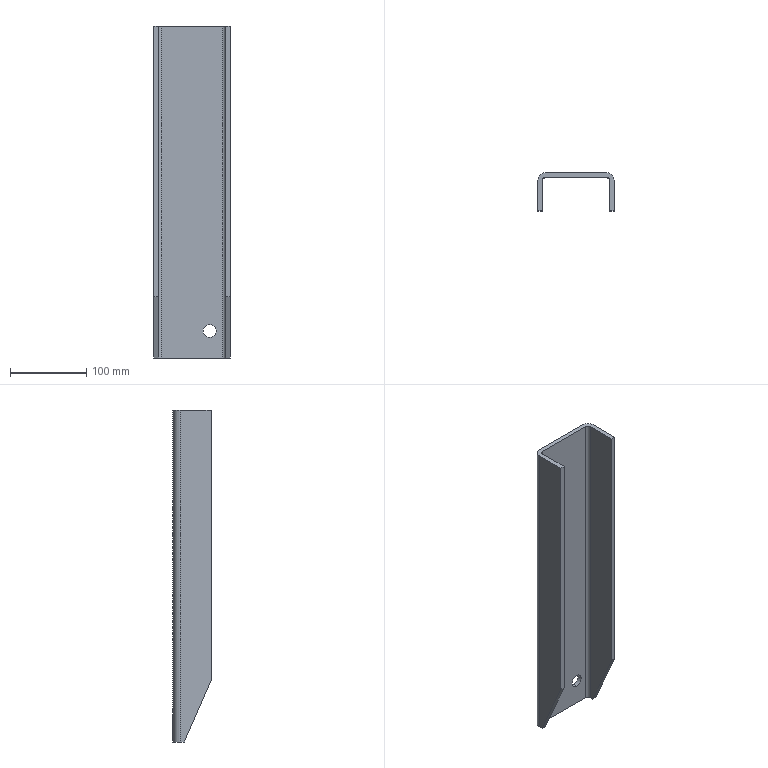Part | SolidWorks | features ICE 2, Extrusion 1 | 1 solid | 18 faces | box 100 x 50 x 435 mm | volume 456835 mm3 | plane 12 | cylinder 6 | commonest cylinder face diameters 8 x2 17 x2 20 x2
STEP:
#1=CARTESIAN_POINT('',(73.2,44.,27.));
#2=VERTEX_POINT('',#1);
#3=CARTESIAN_POINT('',(73.2,44.,44.));
#4=VERTEX_POINT('',#3);
#5=CARTESIAN_POINT('',(73.2,44.,35.5));
#6=DIRECTION('',(0.,1.,0.));
#7=DIRECTION('',(-1.,0.,0.));
#8=AXIS2_PLACEMENT_3D('',#5,#6,#7);
#9=CIRCLE('',#8,8.5);
#10=EDGE_CURVE('',#2,#4,#9,.T.);
#11=ORIENTED_EDGE('',*,*,#10,.F.);
#12=CARTESIAN_POINT('',(73.2,50.,27.));
#13=VERTEX_POINT('',#12);
#14=CARTESIAN_POINT('',(73.2,-385.,27.));
#15=DIRECTION('',(0.,1.,0.));
#16=VECTOR('',#15,1000.);
#17=LINE('',#14,#16);
#18=EDGE_CURVE('',#2,#13,#17,.T.);
#19=ORIENTED_EDGE('',*,*,#18,.T.);
#20=CARTESIAN_POINT('',(73.2,50.,44.));
#21=VERTEX_POINT('',#20);
#22=CARTESIAN_POINT('',(73.2,50.,35.5));
#23=DIRECTION('',(0.,1.,0.));
#24=DIRECTION('',(0.,0.,1.));
#25=AXIS2_PLACEMENT_3D('',#22,#23,#24);
#26=CIRCLE('',#25,8.5);
#27=EDGE_CURVE('',#13,#21,#26,.T.);
#28=ORIENTED_EDGE('',*,*,#27,.T.);
#29=CARTESIAN_POINT('',(73.2,-385.,44.));
#30=DIRECTION('',(0.,1.,0.));
#31=VECTOR('',#30,1000.);
#32=LINE('',#29,#31);
#33=EDGE_CURVE('',#4,#21,#32,.T.);
#34=ORIENTED_EDGE('',*,*,#33,.F.);
#35=EDGE_LOOP('',(#11,#19,#28,#34));
#36=FACE_OUTER_BOUND('',#35,.T.);
#37=CARTESIAN_POINT('',(73.2,-385.,35.5));
#38=DIRECTION('',(0.,1.,0.));
#39=DIRECTION('',(0.,0.,1.));
#40=AXIS2_PLACEMENT_3D('',#37,#38,#39);
#41=CYLINDRICAL_SURFACE('',#40,8.5);
#42=ADVANCED_FACE('',(#36),#41,.F.);
#43=CARTESIAN_POINT('',(100.,35.,0.));
#44=VERTEX_POINT('',#43);
#45=CARTESIAN_POINT('',(100.,0.,80.));
#46=VERTEX_POINT('',#45);
#47=CARTESIAN_POINT('',(100.,0.,80.));
#48=DIRECTION('',(0.,-0.4008,0.9162));
#49=VECTOR('',#48,1000.);
#50=LINE('',#47,#49);
#51=EDGE_CURVE('',#44,#46,#50,.T.);
#52=ORIENTED_EDGE('',*,*,#51,.F.);
#53=CARTESIAN_POINT('',(100.,40.,0.));
#54=VERTEX_POINT('',#53);
#55=CARTESIAN_POINT('',(100.,40.,0.));
#56=DIRECTION('',(0.,-1.,0.));
#57=VECTOR('',#56,1000.);
#58=LINE('',#55,#57);
#59=EDGE_CURVE('',#54,#44,#58,.T.);
#60=ORIENTED_EDGE('',*,*,#59,.F.);
#61=CARTESIAN_POINT('',(100.,40.,435.));
#62=VERTEX_POINT('',#61);
#63=CARTESIAN_POINT('',(100.,40.,435.));
#64=DIRECTION('',(0.,0.,-1.));
#65=VECTOR('',#64,1000.);
#66=LINE('',#63,#65);
#67=EDGE_CURVE('',#62,#54,#66,.T.);
#68=ORIENTED_EDGE('',*,*,#67,.F.);
#69=CARTESIAN_POINT('',(100.,0.,435.));
#70=VERTEX_POINT('',#69);
#71=CARTESIAN_POINT('',(100.,40.,435.));
#72=DIRECTION('',(0.,-1.,0.));
#73=VECTOR('',#72,1000.);
#74=LINE('',#71,#73);
#75=EDGE_CURVE('',#62,#70,#74,.T.);
#76=ORIENTED_EDGE('',*,*,#75,.T.);
#77=CARTESIAN_POINT('',(100.,0.,435.));
#78=DIRECTION('',(0.,0.,-1.));
#79=VECTOR('',#78,1000.);
#80=LINE('',#77,#79);
#81=EDGE_CURVE('',#70,#46,#80,.T.);
#82=ORIENTED_EDGE('',*,*,#81,.T.);
#83=EDGE_LOOP('',(#52,#60,#68,#76,#82));
#84=FACE_OUTER_BOUND('',#83,.T.);
#85=CARTESIAN_POINT('',(100.,40.,435.));
#86=DIRECTION('',(1.,0.,0.));
#87=DIRECTION('',(0.,0.,-1.));
#88=AXIS2_PLACEMENT_3D('',#85,#86,#87);
#89=PLANE('',#88);
#90=ADVANCED_FACE('',(#84),#89,.T.);
#91=CARTESIAN_POINT('',(90.,50.,0.));
#92=VERTEX_POINT('',#91);
#93=CARTESIAN_POINT('',(90.,40.,0.));
#94=DIRECTION('',(0.,0.,-1.));
#95=DIRECTION('',(-1.,0.,0.));
#96=AXIS2_PLACEMENT_3D('',#93,#94,#95);
#97=CIRCLE('',#96,10.);
#98=EDGE_CURVE('',#92,#54,#97,.T.);
#99=ORIENTED_EDGE('',*,*,#98,.F.);
#100=CARTESIAN_POINT('',(90.,50.,435.));
#101=VERTEX_POINT('',#100);
#102=CARTESIAN_POINT('',(90.,50.,435.));
#103=DIRECTION('',(0.,0.,-1.));
#104=VECTOR('',#103,1000.);
#105=LINE('',#102,#104);
#106=EDGE_CURVE('',#101,#92,#105,.T.);
#107=ORIENTED_EDGE('',*,*,#106,.F.);
#108=CARTESIAN_POINT('',(90.,40.,435.));
#109=DIRECTION('',(0.,0.,-1.));
#110=DIRECTION('',(-1.,0.,0.));
#111=AXIS2_PLACEMENT_3D('',#108,#109,#110);
#112=CIRCLE('',#111,10.);
#113=EDGE_CURVE('',#101,#62,#112,.T.);
#114=ORIENTED_EDGE('',*,*,#113,.T.);
#115=ORIENTED_EDGE('',*,*,#67,.T.);
#116=EDGE_LOOP('',(#99,#107,#114,#115));
#117=FACE_OUTER_BOUND('',#116,.T.);
#118=CARTESIAN_POINT('',(90.,40.,435.));
#119=DIRECTION('',(0.,0.,-1.));
#120=DIRECTION('',(-1.,0.,0.));
#121=AXIS2_PLACEMENT_3D('',#118,#119,#120);
#122=CYLINDRICAL_SURFACE('',#121,10.);
#123=ADVANCED_FACE('',(#117),#122,.T.);
#124=CARTESIAN_POINT('',(73.2,50.,35.5));
#125=DIRECTION('',(0.,1.,0.));
#126=DIRECTION('',(0.,0.,1.));
#127=AXIS2_PLACEMENT_3D('',#124,#125,#126);
#128=CIRCLE('',#127,8.5);
#129=EDGE_CURVE('',#21,#13,#128,.T.);
#130=ORIENTED_EDGE('',*,*,#129,.F.);
#131=ORIENTED_EDGE('',*,*,#27,.F.);
#132=EDGE_LOOP('',(#130,#131));
#133=FACE_BOUND('',#132,.T.);
#134=CARTESIAN_POINT('',(10.,50.,0.));
#135=VERTEX_POINT('',#134);
#136=CARTESIAN_POINT('',(10.,50.,0.));
#137=DIRECTION('',(1.,0.,0.));
#138=VECTOR('',#137,1000.);
#139=LINE('',#136,#138);
#140=EDGE_CURVE('',#135,#92,#139,.T.);
#141=ORIENTED_EDGE('',*,*,#140,.F.);
#142=CARTESIAN_POINT('',(10.,50.,435.));
#143=VERTEX_POINT('',#142);
#144=CARTESIAN_POINT('',(10.,50.,435.));
#145=DIRECTION('',(0.,0.,-1.));
#146=VECTOR('',#145,1000.);
#147=LINE('',#144,#146);
#148=EDGE_CURVE('',#143,#135,#147,.T.);
#149=ORIENTED_EDGE('',*,*,#148,.F.);
#150=CARTESIAN_POINT('',(10.,50.,435.));
#151=DIRECTION('',(1.,0.,0.));
#152=VECTOR('',#151,1000.);
#153=LINE('',#150,#152);
#154=EDGE_CURVE('',#143,#101,#153,.T.);
#155=ORIENTED_EDGE('',*,*,#154,.T.);
#156=ORIENTED_EDGE('',*,*,#106,.T.);
#157=EDGE_LOOP('',(#141,#149,#155,#156));
#158=FACE_OUTER_BOUND('',#157,.T.);
#159=CARTESIAN_POINT('',(10.,50.,435.));
#160=DIRECTION('',(0.,1.,0.));
#161=DIRECTION('',(0.,0.,1.));
#162=AXIS2_PLACEMENT_3D('',#159,#160,#161);
#163=PLANE('',#162);
#164=ADVANCED_FACE('',(#133,#158),#163,.T.);
#165=CARTESIAN_POINT('',(0.,40.,0.));
#166=VERTEX_POINT('',#165);
#167=CARTESIAN_POINT('',(10.,40.,0.));
#168=DIRECTION('',(0.,0.,-1.));
#169=DIRECTION('',(-1.,0.,0.));
#170=AXIS2_PLACEMENT_3D('',#167,#168,#169);
#171=CIRCLE('',#170,10.);
#172=EDGE_CURVE('',#166,#135,#171,.T.);
#173=ORIENTED_EDGE('',*,*,#172,.F.);
#174=CARTESIAN_POINT('',(0.,40.,435.));
#175=VERTEX_POINT('',#174);
#176=CARTESIAN_POINT('',(0.,40.,435.));
#177=DIRECTION('',(0.,0.,-1.));
#178=VECTOR('',#177,1000.);
#179=LINE('',#176,#178);
#180=EDGE_CURVE('',#175,#166,#179,.T.);
#181=ORIENTED_EDGE('',*,*,#180,.F.);
#182=CARTESIAN_POINT('',(10.,40.,435.));
#183=DIRECTION('',(0.,0.,-1.));
#184=DIRECTION('',(-1.,0.,0.));
#185=AXIS2_PLACEMENT_3D('',#182,#183,#184);
#186=CIRCLE('',#185,10.);
#187=EDGE_CURVE('',#175,#143,#186,.T.);
#188=ORIENTED_EDGE('',*,*,#187,.T.);
#189=ORIENTED_EDGE('',*,*,#148,.T.);
#190=EDGE_LOOP('',(#173,#181,#188,#189));
#191=FACE_OUTER_BOUND('',#190,.T.);
#192=CARTESIAN_POINT('',(10.,40.,435.));
#193=DIRECTION('',(0.,0.,-1.));
#194=DIRECTION('',(-1.,0.,0.));
#195=AXIS2_PLACEMENT_3D('',#192,#193,#194);
#196=CYLINDRICAL_SURFACE('',#195,10.);
#197=ADVANCED_FACE('',(#191),#196,.T.);
#198=CARTESIAN_POINT('',(0.,0.,80.));
#199=VERTEX_POINT('',#198);
#200=CARTESIAN_POINT('',(0.,35.,0.));
#201=VERTEX_POINT('',#200);
#202=CARTESIAN_POINT('',(0.,-130.361,377.967));
#203=DIRECTION('',(0.,0.4008,-0.9162));
#204=VECTOR('',#203,1000.);
#205=LINE('',#202,#204);
#206=EDGE_CURVE('',#199,#201,#205,.T.);
#207=ORIENTED_EDGE('',*,*,#206,.F.);
#208=CARTESIAN_POINT('',(0.,0.,435.));
#209=VERTEX_POINT('',#208);
#210=CARTESIAN_POINT('',(0.,0.,435.));
#211=DIRECTION('',(0.,0.,-1.));
#212=VECTOR('',#211,1000.);
#213=LINE('',#210,#212);
#214=EDGE_CURVE('',#209,#199,#213,.T.);
#215=ORIENTED_EDGE('',*,*,#214,.F.);
#216=CARTESIAN_POINT('',(0.,0.,435.));
#217=DIRECTION('',(0.,1.,0.));
#218=VECTOR('',#217,1000.);
#219=LINE('',#216,#218);
#220=EDGE_CURVE('',#209,#175,#219,.T.);
#221=ORIENTED_EDGE('',*,*,#220,.T.);
#222=ORIENTED_EDGE('',*,*,#180,.T.);
#223=CARTESIAN_POINT('',(0.,0.,0.));
#224=DIRECTION('',(0.,1.,0.));
#225=VECTOR('',#224,1000.);
#226=LINE('',#223,#225);
#227=EDGE_CURVE('',#201,#166,#226,.T.);
#228=ORIENTED_EDGE('',*,*,#227,.F.);
#229=EDGE_LOOP('',(#207,#215,#221,#222,#228));
#230=FACE_OUTER_BOUND('',#229,.T.);
#231=CARTESIAN_POINT('',(0.,0.,435.));
#232=DIRECTION('',(-1.,0.,0.));
#233=DIRECTION('',(0.,-1.,0.));
#234=AXIS2_PLACEMENT_3D('',#231,#232,#233);
#235=PLANE('',#234);
#236=ADVANCED_FACE('',(#230),#235,.T.);
#237=CARTESIAN_POINT('',(6.,0.,80.));
#238=VERTEX_POINT('',#237);
#239=CARTESIAN_POINT('',(-335.,0.,80.));
#240=DIRECTION('',(1.,0.,0.));
#241=VECTOR('',#240,1000.);
#242=LINE('',#239,#241);
#243=EDGE_CURVE('',#199,#238,#242,.T.);
#244=ORIENTED_EDGE('',*,*,#243,.T.);
#245=CARTESIAN_POINT('',(6.,0.,435.));
#246=VERTEX_POINT('',#245);
#247=CARTESIAN_POINT('',(6.,0.,435.));
#248=DIRECTION('',(0.,0.,-1.));
#249=VECTOR('',#248,1000.);
#250=LINE('',#247,#249);
#251=EDGE_CURVE('',#246,#238,#250,.T.);
#252=ORIENTED_EDGE('',*,*,#251,.F.);
#253=CARTESIAN_POINT('',(6.,0.,435.));
#254=DIRECTION('',(-1.,0.,0.));
#255=VECTOR('',#254,1000.);
#256=LINE('',#253,#255);
#257=EDGE_CURVE('',#246,#209,#256,.T.);
#258=ORIENTED_EDGE('',*,*,#257,.T.);
#259=ORIENTED_EDGE('',*,*,#214,.T.);
#260=EDGE_LOOP('',(#244,#252,#258,#259));
#261=FACE_OUTER_BOUND('',#260,.T.);
#262=CARTESIAN_POINT('',(6.,0.,435.));
#263=DIRECTION('',(0.,-1.,0.));
#264=DIRECTION('',(1.,0.,0.));
#265=AXIS2_PLACEMENT_3D('',#262,#263,#264);
#266=PLANE('',#265);
#267=ADVANCED_FACE('',(#261),#266,.T.);
#268=ORIENTED_EDGE('',*,*,#251,.T.);
#269=CARTESIAN_POINT('',(6.,35.,0.));
#270=VERTEX_POINT('',#269);
#271=CARTESIAN_POINT('',(6.,-130.361,377.967));
#272=DIRECTION('',(0.,0.4008,-0.9162));
#273=VECTOR('',#272,1000.);
#274=LINE('',#271,#273);
#275=EDGE_CURVE('',#238,#270,#274,.T.);
#276=ORIENTED_EDGE('',*,*,#275,.T.);
#277=CARTESIAN_POINT('',(6.,40.,0.));
#278=VERTEX_POINT('',#277);
#279=CARTESIAN_POINT('',(6.,0.,0.));
#280=DIRECTION('',(0.,1.,0.));
#281=VECTOR('',#280,1000.);
#282=LINE('',#279,#281);
#283=EDGE_CURVE('',#270,#278,#282,.T.);
#284=ORIENTED_EDGE('',*,*,#283,.T.);
#285=CARTESIAN_POINT('',(6.,40.,435.));
#286=VERTEX_POINT('',#285);
#287=CARTESIAN_POINT('',(6.,40.,435.));
#288=DIRECTION('',(0.,0.,-1.));
#289=VECTOR('',#288,1000.);
#290=LINE('',#287,#289);
#291=EDGE_CURVE('',#286,#278,#290,.T.);
#292=ORIENTED_EDGE('',*,*,#291,.F.);
#293=CARTESIAN_POINT('',(6.,0.,435.));
#294=DIRECTION('',(0.,1.,0.));
#295=VECTOR('',#294,1000.);
#296=LINE('',#293,#295);
#297=EDGE_CURVE('',#246,#286,#296,.T.);
#298=ORIENTED_EDGE('',*,*,#297,.F.);
#299=EDGE_LOOP('',(#268,#276,#284,#292,#298));
#300=FACE_OUTER_BOUND('',#299,.T.);
#301=CARTESIAN_POINT('',(6.,0.,435.));
#302=DIRECTION('',(-1.,0.,0.));
#303=DIRECTION('',(0.,-1.,0.));
#304=AXIS2_PLACEMENT_3D('',#301,#302,#303);
#305=PLANE('',#304);
#306=ADVANCED_FACE('',(#300),#305,.F.);
#307=CARTESIAN_POINT('',(10.,44.,0.));
#308=VERTEX_POINT('',#307);
#309=CARTESIAN_POINT('',(10.,40.,0.));
#310=DIRECTION('',(0.,0.,-1.));
#311=DIRECTION('',(-1.,0.,0.));
#312=AXIS2_PLACEMENT_3D('',#309,#310,#311);
#313=CIRCLE('',#312,4.);
#314=EDGE_CURVE('',#278,#308,#313,.T.);
#315=ORIENTED_EDGE('',*,*,#314,.T.);
#316=CARTESIAN_POINT('',(10.,44.,435.));
#317=VERTEX_POINT('',#316);
#318=CARTESIAN_POINT('',(10.,44.,435.));
#319=DIRECTION('',(0.,0.,-1.));
#320=VECTOR('',#319,1000.);
#321=LINE('',#318,#320);
#322=EDGE_CURVE('',#317,#308,#321,.T.);
#323=ORIENTED_EDGE('',*,*,#322,.F.);
#324=CARTESIAN_POINT('',(10.,40.,435.));
#325=DIRECTION('',(0.,0.,-1.));
#326=DIRECTION('',(-1.,0.,0.));
#327=AXIS2_PLACEMENT_3D('',#324,#325,#326);
#328=CIRCLE('',#327,4.);
#329=EDGE_CURVE('',#286,#317,#328,.T.);
#330=ORIENTED_EDGE('',*,*,#329,.F.);
#331=ORIENTED_EDGE('',*,*,#291,.T.);
#332=EDGE_LOOP('',(#315,#323,#330,#331));
#333=FACE_OUTER_BOUND('',#332,.T.);
#334=CARTESIAN_POINT('',(10.,40.,435.));
#335=DIRECTION('',(0.,0.,-1.));
#336=DIRECTION('',(-1.,0.,0.));
#337=AXIS2_PLACEMENT_3D('',#334,#335,#336);
#338=CYLINDRICAL_SURFACE('',#337,4.);
#339=ADVANCED_FACE('',(#333),#338,.F.);
#340=CARTESIAN_POINT('',(73.2,44.,35.5));
#341=DIRECTION('',(0.,1.,0.));
#342=DIRECTION('',(-1.,0.,0.));
#343=AXIS2_PLACEMENT_3D('',#340,#341,#342);
#344=CIRCLE('',#343,8.5);
#345=EDGE_CURVE('',#4,#2,#344,.T.);
#346=ORIENTED_EDGE('',*,*,#345,.T.);
#347=ORIENTED_EDGE('',*,*,#10,.T.);
#348=EDGE_LOOP('',(#346,#347));
#349=FACE_BOUND('',#348,.T.);
#350=CARTESIAN_POINT('',(90.,44.,0.));
#351=VERTEX_POINT('',#350);
#352=CARTESIAN_POINT('',(10.,44.,0.));
#353=DIRECTION('',(1.,0.,0.));
#354=VECTOR('',#353,1000.);
#355=LINE('',#352,#354);
#356=EDGE_CURVE('',#308,#351,#355,.T.);
#357=ORIENTED_EDGE('',*,*,#356,.T.);
#358=CARTESIAN_POINT('',(90.,44.,435.));
#359=VERTEX_POINT('',#358);
#360=CARTESIAN_POINT('',(90.,44.,435.));
#361=DIRECTION('',(0.,0.,-1.));
#362=VECTOR('',#361,1000.);
#363=LINE('',#360,#362);
#364=EDGE_CURVE('',#359,#351,#363,.T.);
#365=ORIENTED_EDGE('',*,*,#364,.F.);
#366=CARTESIAN_POINT('',(10.,44.,435.));
#367=DIRECTION('',(1.,0.,0.));
#368=VECTOR('',#367,1000.);
#369=LINE('',#366,#368);
#370=EDGE_CURVE('',#317,#359,#369,.T.);
#371=ORIENTED_EDGE('',*,*,#370,.F.);
#372=ORIENTED_EDGE('',*,*,#322,.T.);
#373=EDGE_LOOP('',(#357,#365,#371,#372));
#374=FACE_OUTER_BOUND('',#373,.T.);
#375=CARTESIAN_POINT('',(10.,44.,435.));
#376=DIRECTION('',(0.,1.,0.));
#377=DIRECTION('',(-1.,0.,0.));
#378=AXIS2_PLACEMENT_3D('',#375,#376,#377);
#379=PLANE('',#378);
#380=ADVANCED_FACE('',(#349,#374),#379,.F.);
#381=CARTESIAN_POINT('',(94.,40.,0.));
#382=VERTEX_POINT('',#381);
#383=CARTESIAN_POINT('',(90.,40.,0.));
#384=DIRECTION('',(0.,0.,-1.));
#385=DIRECTION('',(-1.,0.,0.));
#386=AXIS2_PLACEMENT_3D('',#383,#384,#385);
#387=CIRCLE('',#386,4.);
#388=EDGE_CURVE('',#351,#382,#387,.T.);
#389=ORIENTED_EDGE('',*,*,#388,.T.);
#390=CARTESIAN_POINT('',(94.,40.,435.));
#391=VERTEX_POINT('',#390);
#392=CARTESIAN_POINT('',(94.,40.,435.));
#393=DIRECTION('',(0.,0.,-1.));
#394=VECTOR('',#393,1000.);
#395=LINE('',#392,#394);
#396=EDGE_CURVE('',#391,#382,#395,.T.);
#397=ORIENTED_EDGE('',*,*,#396,.F.);
#398=CARTESIAN_POINT('',(90.,40.,435.));
#399=DIRECTION('',(0.,0.,-1.));
#400=DIRECTION('',(-1.,0.,0.));
#401=AXIS2_PLACEMENT_3D('',#398,#399,#400);
#402=CIRCLE('',#401,4.);
#403=EDGE_CURVE('',#359,#391,#402,.T.);
#404=ORIENTED_EDGE('',*,*,#403,.F.);
#405=ORIENTED_EDGE('',*,*,#364,.T.);
#406=EDGE_LOOP('',(#389,#397,#404,#405));
#407=FACE_OUTER_BOUND('',#406,.T.);
#408=CARTESIAN_POINT('',(90.,40.,435.));
#409=DIRECTION('',(0.,0.,-1.));
#410=DIRECTION('',(-1.,0.,0.));
#411=AXIS2_PLACEMENT_3D('',#408,#409,#410);
#412=CYLINDRICAL_SURFACE('',#411,4.);
#413=ADVANCED_FACE('',(#407),#412,.F.);
#414=CARTESIAN_POINT('',(94.,35.,0.));
#415=VERTEX_POINT('',#414);
#416=CARTESIAN_POINT('',(94.,40.,0.));
#417=DIRECTION('',(0.,-1.,0.));
#418=VECTOR('',#417,1000.);
#419=LINE('',#416,#418);
#420=EDGE_CURVE('',#382,#415,#419,.T.);
#421=ORIENTED_EDGE('',*,*,#420,.T.);
#422=CARTESIAN_POINT('',(94.,0.,80.));
#423=VERTEX_POINT('',#422);
#424=CARTESIAN_POINT('',(94.,-123.934,363.279));
#425=DIRECTION('',(0.,-0.4008,0.9162));
#426=VECTOR('',#425,1000.);
#427=LINE('',#424,#426);
#428=EDGE_CURVE('',#415,#423,#427,.T.);
#429=ORIENTED_EDGE('',*,*,#428,.T.);
#430=CARTESIAN_POINT('',(94.,0.,435.));
#431=VERTEX_POINT('',#430);
#432=CARTESIAN_POINT('',(94.,0.,435.));
#433=DIRECTION('',(0.,0.,-1.));
#434=VECTOR('',#433,1000.);
#435=LINE('',#432,#434);
#436=EDGE_CURVE('',#431,#423,#435,.T.);
#437=ORIENTED_EDGE('',*,*,#436,.F.);
#438=CARTESIAN_POINT('',(94.,40.,435.));
#439=DIRECTION('',(0.,-1.,0.));
#440=VECTOR('',#439,1000.);
#441=LINE('',#438,#440);
#442=EDGE_CURVE('',#391,#431,#441,.T.);
#443=ORIENTED_EDGE('',*,*,#442,.F.);
#444=ORIENTED_EDGE('',*,*,#396,.T.);
#445=EDGE_LOOP('',(#421,#429,#437,#443,#444));
#446=FACE_OUTER_BOUND('',#445,.T.);
#447=CARTESIAN_POINT('',(94.,40.,435.));
#448=DIRECTION('',(1.,0.,0.));
#449=DIRECTION('',(0.,1.,0.));
#450=AXIS2_PLACEMENT_3D('',#447,#448,#449);
#451=PLANE('',#450);
#452=ADVANCED_FACE('',(#446),#451,.F.);
#453=CARTESIAN_POINT('',(-335.,0.,80.));
#454=DIRECTION('',(1.,0.,0.));
#455=VECTOR('',#454,1000.);
#456=LINE('',#453,#455);
#457=EDGE_CURVE('',#423,#46,#456,.T.);
#458=ORIENTED_EDGE('',*,*,#457,.T.);
#459=ORIENTED_EDGE('',*,*,#81,.F.);
#460=CARTESIAN_POINT('',(100.,0.,435.));
#461=DIRECTION('',(-1.,0.,0.));
#462=VECTOR('',#461,1000.);
#463=LINE('',#460,#462);
#464=EDGE_CURVE('',#70,#431,#463,.T.);
#465=ORIENTED_EDGE('',*,*,#464,.T.);
#466=ORIENTED_EDGE('',*,*,#436,.T.);
#467=EDGE_LOOP('',(#458,#459,#465,#466));
#468=FACE_OUTER_BOUND('',#467,.T.);
#469=CARTESIAN_POINT('',(100.,0.,435.));
#470=DIRECTION('',(0.,-1.,0.));
#471=DIRECTION('',(0.,0.,-1.));
#472=AXIS2_PLACEMENT_3D('',#469,#470,#471);
#473=PLANE('',#472);
#474=ADVANCED_FACE('',(#468),#473,.T.);
#475=ORIENTED_EDGE('',*,*,#75,.F.);
#476=ORIENTED_EDGE('',*,*,#113,.F.);
#477=ORIENTED_EDGE('',*,*,#154,.F.);
#478=ORIENTED_EDGE('',*,*,#187,.F.);
#479=ORIENTED_EDGE('',*,*,#220,.F.);
#480=ORIENTED_EDGE('',*,*,#257,.F.);
#481=ORIENTED_EDGE('',*,*,#297,.T.);
#482=ORIENTED_EDGE('',*,*,#329,.T.);
#483=ORIENTED_EDGE('',*,*,#370,.T.);
#484=ORIENTED_EDGE('',*,*,#403,.T.);
#485=ORIENTED_EDGE('',*,*,#442,.T.);
#486=ORIENTED_EDGE('',*,*,#464,.F.);
#487=EDGE_LOOP('',(#475,#476,#477,#478,#479,#480,#481,#482,#483,#484,#485,#486));
#488=FACE_OUTER_BOUND('',#487,.T.);
#489=CARTESIAN_POINT('',(90.,40.,435.));
#490=DIRECTION('',(0.,0.,-1.));
#491=DIRECTION('',(-1.,0.,0.));
#492=AXIS2_PLACEMENT_3D('',#489,#490,#491);
#493=PLANE('',#492);
#494=ADVANCED_FACE('',(#488),#493,.F.);
#495=CARTESIAN_POINT('',(90.,35.,0.));
#496=DIRECTION('',(1.,0.,0.));
#497=VECTOR('',#496,1000.);
#498=LINE('',#495,#497);
#499=EDGE_CURVE('',#201,#270,#498,.T.);
#500=ORIENTED_EDGE('',*,*,#499,.F.);
#501=ORIENTED_EDGE('',*,*,#227,.T.);
#502=ORIENTED_EDGE('',*,*,#172,.T.);
#503=ORIENTED_EDGE('',*,*,#140,.T.);
#504=ORIENTED_EDGE('',*,*,#98,.T.);
#505=ORIENTED_EDGE('',*,*,#59,.T.);
#506=CARTESIAN_POINT('',(90.,35.,0.));
#507=DIRECTION('',(1.,0.,0.));
#508=VECTOR('',#507,1000.);
#509=LINE('',#506,#508);
#510=EDGE_CURVE('',#415,#44,#509,.T.);
#511=ORIENTED_EDGE('',*,*,#510,.F.);
#512=ORIENTED_EDGE('',*,*,#420,.F.);
#513=ORIENTED_EDGE('',*,*,#388,.F.);
#514=ORIENTED_EDGE('',*,*,#356,.F.);
#515=ORIENTED_EDGE('',*,*,#314,.F.);
#516=ORIENTED_EDGE('',*,*,#283,.F.);
#517=EDGE_LOOP('',(#500,#501,#502,#503,#504,#505,#511,#512,#513,#514,#515,#516));
#518=FACE_OUTER_BOUND('',#517,.T.);
#519=CARTESIAN_POINT('',(90.,40.,0.));
#520=DIRECTION('',(0.,0.,-1.));
#521=DIRECTION('',(-1.,0.,0.));
#522=AXIS2_PLACEMENT_3D('',#519,#520,#521);
#523=PLANE('',#522);
#524=ADVANCED_FACE('',(#518),#523,.T.);
#525=ORIENTED_EDGE('',*,*,#18,.F.);
#526=ORIENTED_EDGE('',*,*,#345,.F.);
#527=ORIENTED_EDGE('',*,*,#33,.T.);
#528=ORIENTED_EDGE('',*,*,#129,.T.);
#529=EDGE_LOOP('',(#525,#526,#527,#528));
#530=FACE_OUTER_BOUND('',#529,.T.);
#531=CARTESIAN_POINT('',(73.2,-385.,35.5));
#532=DIRECTION('',(0.,1.,0.));
#533=DIRECTION('',(0.,0.,1.));
#534=AXIS2_PLACEMENT_3D('',#531,#532,#533);
#535=CYLINDRICAL_SURFACE('',#534,8.5);
#536=ADVANCED_FACE('',(#530),#535,.F.);
#537=ORIENTED_EDGE('',*,*,#510,.T.);
#538=ORIENTED_EDGE('',*,*,#51,.T.);
#539=ORIENTED_EDGE('',*,*,#457,.F.);
#540=ORIENTED_EDGE('',*,*,#428,.F.);
#541=EDGE_LOOP('',(#537,#538,#539,#540));
#542=FACE_OUTER_BOUND('',#541,.T.);
#543=CARTESIAN_POINT('',(-335.,0.,80.));
#544=DIRECTION('',(0.,0.9162,0.4008));
#545=DIRECTION('',(0.,-0.4008,0.9162));
#546=AXIS2_PLACEMENT_3D('',#543,#544,#545);
#547=PLANE('',#546);
#548=ADVANCED_FACE('',(#542),#547,.F.);
#549=ORIENTED_EDGE('',*,*,#206,.T.);
#550=ORIENTED_EDGE('',*,*,#499,.T.);
#551=ORIENTED_EDGE('',*,*,#275,.F.);
#552=ORIENTED_EDGE('',*,*,#243,.F.);
#553=EDGE_LOOP('',(#549,#550,#551,#552));
#554=FACE_OUTER_BOUND('',#553,.T.);
#555=CARTESIAN_POINT('',(-335.,0.,80.));
#556=DIRECTION('',(0.,0.9162,0.4008));
#557=DIRECTION('',(0.,-0.4008,0.9162));
#558=AXIS2_PLACEMENT_3D('',#555,#556,#557);
#559=PLANE('',#558);
#560=ADVANCED_FACE('',(#554),#559,.F.);
#561=CLOSED_SHELL('',(#42,#90,#123,#164,#197,#236,#267,#306,#339,#380,#413,#452,#474,#494,#524,#536,#548,#560));
#562=MANIFOLD_SOLID_BREP('',#561);
#563=CARTESIAN_POINT('',(0.,0.,0.));
#564=DIRECTION('',(0.,0.,1.));
#565=DIRECTION('',(1.,0.,0.));
#566=AXIS2_PLACEMENT_3D('',#563,#564,#565);
#567=(LENGTH_UNIT()NAMED_UNIT(*)SI_UNIT(.MILLI.,.METRE.));
#568=UNCERTAINTY_MEASURE_WITH_UNIT(LENGTH_MEASURE(0.00001),#567,'','');
#569=(NAMED_UNIT(*)PLANE_ANGLE_UNIT()SI_UNIT($,.RADIAN.));
#570=(NAMED_UNIT(*)SI_UNIT($,.STERADIAN.)SOLID_ANGLE_UNIT());
#571=(GEOMETRIC_REPRESENTATION_CONTEXT(3)GLOBAL_UNCERTAINTY_ASSIGNED_CONTEXT((#568))GLOBAL_UNIT_ASSIGNED_CONTEXT((#567,#569,#570))REPRESENTATION_CONTEXT('',''));
#572=ADVANCED_BREP_SHAPE_REPRESENTATION('',(#562,#566),#571);